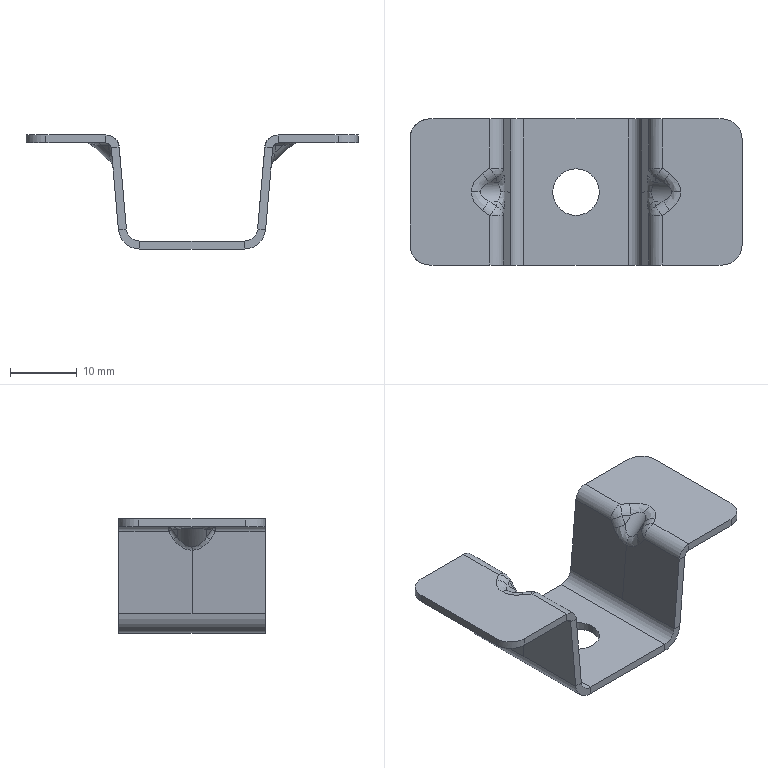Part | 1 solid | 106 faces | box 49.915 x 21.985 x 17.167 mm | volume 1952 mm3 | cylinder 40 | plane 30 | spline 28 | sphere 8 | commonest cylinder face diameters 4 x16 1.6 x12 6 x4 6.4 x4 7 x4